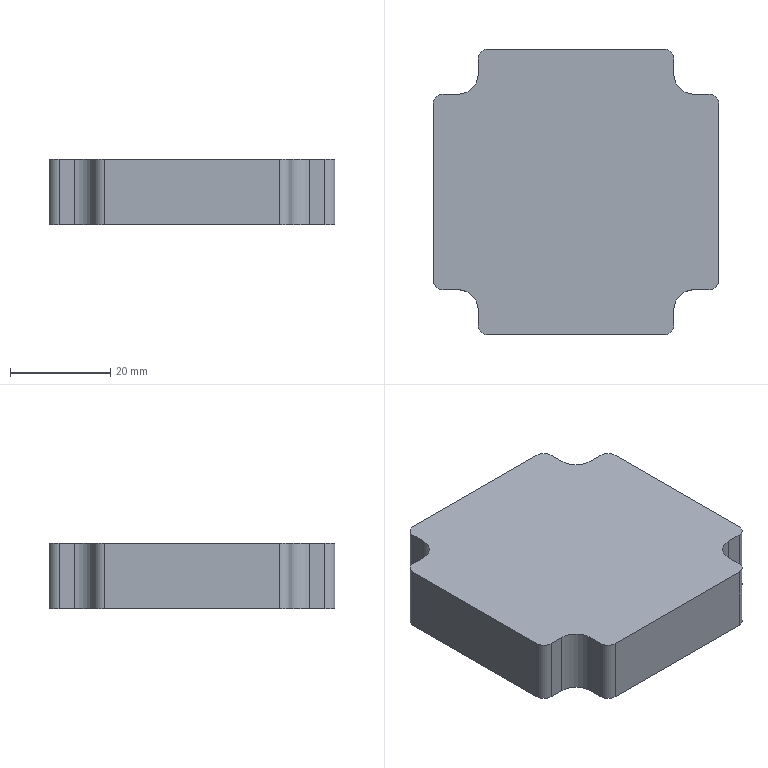Part | SolidWorks | features BaseBody 1 | 1 solid | 41 faces | box 57 x 57 x 13 mm | volume 37451 mm3 | cylinder 22 | plane 19 | commonest cylinder face diameters 3 x8 4 x8 8 x4 10 x2
STEP:
#1=CARTESIAN_POINT('',(5.,0.,7.));
#2=VERTEX_POINT('',#1);
#3=CARTESIAN_POINT('',(-5.,0.,7.));
#4=VERTEX_POINT('',#3);
#5=CARTESIAN_POINT('',(0.,0.,7.));
#6=DIRECTION('',(0.,0.,-1.));
#7=DIRECTION('',(-1.,0.,0.));
#8=AXIS2_PLACEMENT_3D('',#5,#6,#7);
#9=CIRCLE('',#8,5.);
#10=EDGE_CURVE('',#2,#4,#9,.T.);
#11=ORIENTED_EDGE('',*,*,#10,.F.);
#12=CARTESIAN_POINT('',(5.,0.,0.));
#13=VERTEX_POINT('',#12);
#14=CARTESIAN_POINT('',(5.,0.,7.));
#15=DIRECTION('',(0.,0.,-1.));
#16=VECTOR('',#15,1000.);
#17=LINE('',#14,#16);
#18=EDGE_CURVE('',#2,#13,#17,.T.);
#19=ORIENTED_EDGE('',*,*,#18,.T.);
#20=CARTESIAN_POINT('',(-5.,0.,0.));
#21=VERTEX_POINT('',#20);
#22=CARTESIAN_POINT('',(0.,0.,0.));
#23=DIRECTION('',(0.,0.,-1.));
#24=DIRECTION('',(-1.,0.,0.));
#25=AXIS2_PLACEMENT_3D('',#22,#23,#24);
#26=CIRCLE('',#25,5.);
#27=EDGE_CURVE('',#13,#21,#26,.T.);
#28=ORIENTED_EDGE('',*,*,#27,.T.);
#29=CARTESIAN_POINT('',(-5.,0.,7.));
#30=DIRECTION('',(0.,0.,-1.));
#31=VECTOR('',#30,1000.);
#32=LINE('',#29,#31);
#33=EDGE_CURVE('',#4,#21,#32,.T.);
#34=ORIENTED_EDGE('',*,*,#33,.F.);
#35=EDGE_LOOP('',(#11,#19,#28,#34));
#36=FACE_OUTER_BOUND('',#35,.T.);
#37=CARTESIAN_POINT('',(0.,0.,7.));
#38=DIRECTION('',(0.,0.,-1.));
#39=DIRECTION('',(-1.,0.,0.));
#40=AXIS2_PLACEMENT_3D('',#37,#38,#39);
#41=CYLINDRICAL_SURFACE('',#40,5.);
#42=ADVANCED_FACE('',(#36),#41,.F.);
#43=CARTESIAN_POINT('',(-24.,-16.5,4.));
#44=VERTEX_POINT('',#43);
#45=CARTESIAN_POINT('',(-27.,-16.5,4.));
#46=VERTEX_POINT('',#45);
#47=CARTESIAN_POINT('',(-25.5,-16.5,4.));
#48=DIRECTION('',(0.,0.,-1.));
#49=DIRECTION('',(-1.,0.,0.));
#50=AXIS2_PLACEMENT_3D('',#47,#48,#49);
#51=CIRCLE('',#50,1.5);
#52=EDGE_CURVE('',#44,#46,#51,.T.);
#53=ORIENTED_EDGE('',*,*,#52,.F.);
#54=CARTESIAN_POINT('',(-24.,-16.5,0.));
#55=VERTEX_POINT('',#54);
#56=CARTESIAN_POINT('',(-24.,-16.5,4.));
#57=DIRECTION('',(0.,0.,-1.));
#58=VECTOR('',#57,1000.);
#59=LINE('',#56,#58);
#60=EDGE_CURVE('',#44,#55,#59,.T.);
#61=ORIENTED_EDGE('',*,*,#60,.T.);
#62=CARTESIAN_POINT('',(-27.,-16.5,0.));
#63=VERTEX_POINT('',#62);
#64=CARTESIAN_POINT('',(-25.5,-16.5,0.));
#65=DIRECTION('',(0.,0.,-1.));
#66=DIRECTION('',(-1.,0.,0.));
#67=AXIS2_PLACEMENT_3D('',#64,#65,#66);
#68=CIRCLE('',#67,1.5);
#69=EDGE_CURVE('',#55,#63,#68,.T.);
#70=ORIENTED_EDGE('',*,*,#69,.T.);
#71=CARTESIAN_POINT('',(-27.,-16.5,4.));
#72=DIRECTION('',(0.,0.,-1.));
#73=VECTOR('',#72,1000.);
#74=LINE('',#71,#73);
#75=EDGE_CURVE('',#46,#63,#74,.T.);
#76=ORIENTED_EDGE('',*,*,#75,.F.);
#77=EDGE_LOOP('',(#53,#61,#70,#76));
#78=FACE_OUTER_BOUND('',#77,.T.);
#79=CARTESIAN_POINT('',(-25.5,-16.5,4.));
#80=DIRECTION('',(0.,0.,-1.));
#81=DIRECTION('',(-1.,0.,0.));
#82=AXIS2_PLACEMENT_3D('',#79,#80,#81);
#83=CYLINDRICAL_SURFACE('',#82,1.5);
#84=ADVANCED_FACE('',(#78),#83,.F.);
#85=CARTESIAN_POINT('',(-15.,25.5,4.));
#86=VERTEX_POINT('',#85);
#87=CARTESIAN_POINT('',(-18.,25.5,4.));
#88=VERTEX_POINT('',#87);
#89=CARTESIAN_POINT('',(-16.5,25.5,4.));
#90=DIRECTION('',(0.,0.,-1.));
#91=DIRECTION('',(-1.,0.,0.));
#92=AXIS2_PLACEMENT_3D('',#89,#90,#91);
#93=CIRCLE('',#92,1.5);
#94=EDGE_CURVE('',#86,#88,#93,.T.);
#95=ORIENTED_EDGE('',*,*,#94,.F.);
#96=CARTESIAN_POINT('',(-15.,25.5,0.));
#97=VERTEX_POINT('',#96);
#98=CARTESIAN_POINT('',(-15.,25.5,4.));
#99=DIRECTION('',(0.,0.,-1.));
#100=VECTOR('',#99,1000.);
#101=LINE('',#98,#100);
#102=EDGE_CURVE('',#86,#97,#101,.T.);
#103=ORIENTED_EDGE('',*,*,#102,.T.);
#104=CARTESIAN_POINT('',(-18.,25.5,0.));
#105=VERTEX_POINT('',#104);
#106=CARTESIAN_POINT('',(-16.5,25.5,0.));
#107=DIRECTION('',(0.,0.,-1.));
#108=DIRECTION('',(-1.,0.,0.));
#109=AXIS2_PLACEMENT_3D('',#106,#107,#108);
#110=CIRCLE('',#109,1.5);
#111=EDGE_CURVE('',#97,#105,#110,.T.);
#112=ORIENTED_EDGE('',*,*,#111,.T.);
#113=CARTESIAN_POINT('',(-18.,25.5,4.));
#114=DIRECTION('',(0.,0.,-1.));
#115=VECTOR('',#114,1000.);
#116=LINE('',#113,#115);
#117=EDGE_CURVE('',#88,#105,#116,.T.);
#118=ORIENTED_EDGE('',*,*,#117,.F.);
#119=EDGE_LOOP('',(#95,#103,#112,#118));
#120=FACE_OUTER_BOUND('',#119,.T.);
#121=CARTESIAN_POINT('',(-16.5,25.5,4.));
#122=DIRECTION('',(0.,0.,-1.));
#123=DIRECTION('',(-1.,0.,0.));
#124=AXIS2_PLACEMENT_3D('',#121,#122,#123);
#125=CYLINDRICAL_SURFACE('',#124,1.5);
#126=ADVANCED_FACE('',(#120),#125,.F.);
#127=CARTESIAN_POINT('',(27.,16.5,4.));
#128=VERTEX_POINT('',#127);
#129=CARTESIAN_POINT('',(24.,16.5,4.));
#130=VERTEX_POINT('',#129);
#131=CARTESIAN_POINT('',(25.5,16.5,4.));
#132=DIRECTION('',(0.,0.,-1.));
#133=DIRECTION('',(-1.,0.,0.));
#134=AXIS2_PLACEMENT_3D('',#131,#132,#133);
#135=CIRCLE('',#134,1.5);
#136=EDGE_CURVE('',#128,#130,#135,.T.);
#137=ORIENTED_EDGE('',*,*,#136,.F.);
#138=CARTESIAN_POINT('',(27.,16.5,0.));
#139=VERTEX_POINT('',#138);
#140=CARTESIAN_POINT('',(27.,16.5,4.));
#141=DIRECTION('',(0.,0.,-1.));
#142=VECTOR('',#141,1000.);
#143=LINE('',#140,#142);
#144=EDGE_CURVE('',#128,#139,#143,.T.);
#145=ORIENTED_EDGE('',*,*,#144,.T.);
#146=CARTESIAN_POINT('',(24.,16.5,0.));
#147=VERTEX_POINT('',#146);
#148=CARTESIAN_POINT('',(25.5,16.5,0.));
#149=DIRECTION('',(0.,0.,-1.));
#150=DIRECTION('',(-1.,0.,0.));
#151=AXIS2_PLACEMENT_3D('',#148,#149,#150);
#152=CIRCLE('',#151,1.5);
#153=EDGE_CURVE('',#139,#147,#152,.T.);
#154=ORIENTED_EDGE('',*,*,#153,.T.);
#155=CARTESIAN_POINT('',(24.,16.5,4.));
#156=DIRECTION('',(0.,0.,-1.));
#157=VECTOR('',#156,1000.);
#158=LINE('',#155,#157);
#159=EDGE_CURVE('',#130,#147,#158,.T.);
#160=ORIENTED_EDGE('',*,*,#159,.F.);
#161=EDGE_LOOP('',(#137,#145,#154,#160));
#162=FACE_OUTER_BOUND('',#161,.T.);
#163=CARTESIAN_POINT('',(25.5,16.5,4.));
#164=DIRECTION('',(0.,0.,-1.));
#165=DIRECTION('',(-1.,0.,0.));
#166=AXIS2_PLACEMENT_3D('',#163,#164,#165);
#167=CYLINDRICAL_SURFACE('',#166,1.5);
#168=ADVANCED_FACE('',(#162),#167,.F.);
#169=CARTESIAN_POINT('',(18.,-25.5,4.));
#170=VERTEX_POINT('',#169);
#171=CARTESIAN_POINT('',(15.,-25.5,4.));
#172=VERTEX_POINT('',#171);
#173=CARTESIAN_POINT('',(16.5,-25.5,4.));
#174=DIRECTION('',(0.,0.,-1.));
#175=DIRECTION('',(-1.,0.,0.));
#176=AXIS2_PLACEMENT_3D('',#173,#174,#175);
#177=CIRCLE('',#176,1.5);
#178=EDGE_CURVE('',#170,#172,#177,.T.);
#179=ORIENTED_EDGE('',*,*,#178,.F.);
#180=CARTESIAN_POINT('',(18.,-25.5,0.));
#181=VERTEX_POINT('',#180);
#182=CARTESIAN_POINT('',(18.,-25.5,4.));
#183=DIRECTION('',(0.,0.,-1.));
#184=VECTOR('',#183,1000.);
#185=LINE('',#182,#184);
#186=EDGE_CURVE('',#170,#181,#185,.T.);
#187=ORIENTED_EDGE('',*,*,#186,.T.);
#188=CARTESIAN_POINT('',(15.,-25.5,0.));
#189=VERTEX_POINT('',#188);
#190=CARTESIAN_POINT('',(16.5,-25.5,0.));
#191=DIRECTION('',(0.,0.,-1.));
#192=DIRECTION('',(-1.,0.,0.));
#193=AXIS2_PLACEMENT_3D('',#190,#191,#192);
#194=CIRCLE('',#193,1.5);
#195=EDGE_CURVE('',#181,#189,#194,.T.);
#196=ORIENTED_EDGE('',*,*,#195,.T.);
#197=CARTESIAN_POINT('',(15.,-25.5,4.));
#198=DIRECTION('',(0.,0.,-1.));
#199=VECTOR('',#198,1000.);
#200=LINE('',#197,#199);
#201=EDGE_CURVE('',#172,#189,#200,.T.);
#202=ORIENTED_EDGE('',*,*,#201,.F.);
#203=EDGE_LOOP('',(#179,#187,#196,#202));
#204=FACE_OUTER_BOUND('',#203,.T.);
#205=CARTESIAN_POINT('',(16.5,-25.5,4.));
#206=DIRECTION('',(0.,0.,-1.));
#207=DIRECTION('',(-1.,0.,0.));
#208=AXIS2_PLACEMENT_3D('',#205,#206,#207);
#209=CYLINDRICAL_SURFACE('',#208,1.5);
#210=ADVANCED_FACE('',(#204),#209,.F.);
#211=CARTESIAN_POINT('',(19.5,26.5,0.));
#212=VERTEX_POINT('',#211);
#213=CARTESIAN_POINT('',(17.5,28.5,0.));
#214=VERTEX_POINT('',#213);
#215=CARTESIAN_POINT('',(17.5,26.5,0.));
#216=DIRECTION('',(0.,0.,1.));
#217=DIRECTION('',(-1.,0.,0.));
#218=AXIS2_PLACEMENT_3D('',#215,#216,#217);
#219=CIRCLE('',#218,2.);
#220=EDGE_CURVE('',#212,#214,#219,.T.);
#221=ORIENTED_EDGE('',*,*,#220,.T.);
#222=CARTESIAN_POINT('',(17.5,28.5,13.));
#223=VERTEX_POINT('',#222);
#224=CARTESIAN_POINT('',(17.5,28.5,13.));
#225=DIRECTION('',(0.,0.,-1.));
#226=VECTOR('',#225,1000.);
#227=LINE('',#224,#226);
#228=EDGE_CURVE('',#223,#214,#227,.T.);
#229=ORIENTED_EDGE('',*,*,#228,.F.);
#230=CARTESIAN_POINT('',(19.5,26.5,13.));
#231=VERTEX_POINT('',#230);
#232=CARTESIAN_POINT('',(17.5,26.5,13.));
#233=DIRECTION('',(0.,0.,1.));
#234=DIRECTION('',(-1.,0.,0.));
#235=AXIS2_PLACEMENT_3D('',#232,#233,#234);
#236=CIRCLE('',#235,2.);
#237=EDGE_CURVE('',#231,#223,#236,.T.);
#238=ORIENTED_EDGE('',*,*,#237,.F.);
#239=CARTESIAN_POINT('',(19.5,26.5,13.));
#240=DIRECTION('',(0.,0.,-1.));
#241=VECTOR('',#240,1000.);
#242=LINE('',#239,#241);
#243=EDGE_CURVE('',#231,#212,#242,.T.);
#244=ORIENTED_EDGE('',*,*,#243,.T.);
#245=EDGE_LOOP('',(#221,#229,#238,#244));
#246=FACE_OUTER_BOUND('',#245,.T.);
#247=CARTESIAN_POINT('',(17.5,26.5,13.));
#248=DIRECTION('',(0.,0.,-1.));
#249=DIRECTION('',(-1.,0.,0.));
#250=AXIS2_PLACEMENT_3D('',#247,#248,#249);
#251=CYLINDRICAL_SURFACE('',#250,2.);
#252=ADVANCED_FACE('',(#246),#251,.T.);
#253=CARTESIAN_POINT('',(-17.5,28.5,0.));
#254=VERTEX_POINT('',#253);
#255=CARTESIAN_POINT('',(-17.5,28.5,0.));
#256=DIRECTION('',(-1.,0.,0.));
#257=VECTOR('',#256,1000.);
#258=LINE('',#255,#257);
#259=EDGE_CURVE('',#214,#254,#258,.T.);
#260=ORIENTED_EDGE('',*,*,#259,.T.);
#261=CARTESIAN_POINT('',(-17.5,28.5,13.));
#262=VERTEX_POINT('',#261);
#263=CARTESIAN_POINT('',(-17.5,28.5,13.));
#264=DIRECTION('',(0.,0.,-1.));
#265=VECTOR('',#264,1000.);
#266=LINE('',#263,#265);
#267=EDGE_CURVE('',#262,#254,#266,.T.);
#268=ORIENTED_EDGE('',*,*,#267,.F.);
#269=CARTESIAN_POINT('',(-17.5,28.5,13.));
#270=DIRECTION('',(-1.,0.,0.));
#271=VECTOR('',#270,1000.);
#272=LINE('',#269,#271);
#273=EDGE_CURVE('',#223,#262,#272,.T.);
#274=ORIENTED_EDGE('',*,*,#273,.F.);
#275=ORIENTED_EDGE('',*,*,#228,.T.);
#276=EDGE_LOOP('',(#260,#268,#274,#275));
#277=FACE_OUTER_BOUND('',#276,.T.);
#278=CARTESIAN_POINT('',(-17.5,28.5,13.));
#279=DIRECTION('',(0.,-1.,0.));
#280=DIRECTION('',(0.,0.,-1.));
#281=AXIS2_PLACEMENT_3D('',#278,#279,#280);
#282=PLANE('',#281);
#283=ADVANCED_FACE('',(#277),#282,.F.);
#284=CARTESIAN_POINT('',(-19.5,26.5,0.));
#285=VERTEX_POINT('',#284);
#286=CARTESIAN_POINT('',(-17.5,26.5,0.));
#287=DIRECTION('',(0.,0.,1.));
#288=DIRECTION('',(-1.,0.,0.));
#289=AXIS2_PLACEMENT_3D('',#286,#287,#288);
#290=CIRCLE('',#289,2.);
#291=EDGE_CURVE('',#254,#285,#290,.T.);
#292=ORIENTED_EDGE('',*,*,#291,.T.);
#293=CARTESIAN_POINT('',(-19.5,26.5,13.));
#294=VERTEX_POINT('',#293);
#295=CARTESIAN_POINT('',(-19.5,26.5,13.));
#296=DIRECTION('',(0.,0.,-1.));
#297=VECTOR('',#296,1000.);
#298=LINE('',#295,#297);
#299=EDGE_CURVE('',#294,#285,#298,.T.);
#300=ORIENTED_EDGE('',*,*,#299,.F.);
#301=CARTESIAN_POINT('',(-17.5,26.5,13.));
#302=DIRECTION('',(0.,0.,1.));
#303=DIRECTION('',(-1.,0.,0.));
#304=AXIS2_PLACEMENT_3D('',#301,#302,#303);
#305=CIRCLE('',#304,2.);
#306=EDGE_CURVE('',#262,#294,#305,.T.);
#307=ORIENTED_EDGE('',*,*,#306,.F.);
#308=ORIENTED_EDGE('',*,*,#267,.T.);
#309=EDGE_LOOP('',(#292,#300,#307,#308));
#310=FACE_OUTER_BOUND('',#309,.T.);
#311=CARTESIAN_POINT('',(-17.5,26.5,13.));
#312=DIRECTION('',(0.,0.,-1.));
#313=DIRECTION('',(-1.,0.,0.));
#314=AXIS2_PLACEMENT_3D('',#311,#312,#313);
#315=CYLINDRICAL_SURFACE('',#314,2.);
#316=ADVANCED_FACE('',(#310),#315,.T.);
#317=CARTESIAN_POINT('',(-19.5,23.5,0.));
#318=VERTEX_POINT('',#317);
#319=CARTESIAN_POINT('',(-19.5,23.5,0.));
#320=DIRECTION('',(0.,-1.,0.));
#321=VECTOR('',#320,1000.);
#322=LINE('',#319,#321);
#323=EDGE_CURVE('',#285,#318,#322,.T.);
#324=ORIENTED_EDGE('',*,*,#323,.T.);
#325=CARTESIAN_POINT('',(-19.5,23.5,13.));
#326=VERTEX_POINT('',#325);
#327=CARTESIAN_POINT('',(-19.5,23.5,13.));
#328=DIRECTION('',(0.,0.,-1.));
#329=VECTOR('',#328,1000.);
#330=LINE('',#327,#329);
#331=EDGE_CURVE('',#326,#318,#330,.T.);
#332=ORIENTED_EDGE('',*,*,#331,.F.);
#333=CARTESIAN_POINT('',(-19.5,23.5,13.));
#334=DIRECTION('',(0.,-1.,0.));
#335=VECTOR('',#334,1000.);
#336=LINE('',#333,#335);
#337=EDGE_CURVE('',#294,#326,#336,.T.);
#338=ORIENTED_EDGE('',*,*,#337,.F.);
#339=ORIENTED_EDGE('',*,*,#299,.T.);
#340=EDGE_LOOP('',(#324,#332,#338,#339));
#341=FACE_OUTER_BOUND('',#340,.T.);
#342=CARTESIAN_POINT('',(-19.5,23.5,13.));
#343=DIRECTION('',(1.,0.,0.));
#344=DIRECTION('',(0.,1.,0.));
#345=AXIS2_PLACEMENT_3D('',#342,#343,#344);
#346=PLANE('',#345);
#347=ADVANCED_FACE('',(#341),#346,.F.);
#348=CARTESIAN_POINT('',(-23.5,19.5,0.));
#349=VERTEX_POINT('',#348);
#350=CARTESIAN_POINT('',(-23.5,23.5,0.));
#351=DIRECTION('',(0.,0.,-1.));
#352=DIRECTION('',(1.,0.,0.));
#353=AXIS2_PLACEMENT_3D('',#350,#351,#352);
#354=CIRCLE('',#353,4.);
#355=EDGE_CURVE('',#318,#349,#354,.T.);
#356=ORIENTED_EDGE('',*,*,#355,.T.);
#357=CARTESIAN_POINT('',(-23.5,19.5,13.));
#358=VERTEX_POINT('',#357);
#359=CARTESIAN_POINT('',(-23.5,19.5,13.));
#360=DIRECTION('',(0.,0.,-1.));
#361=VECTOR('',#360,1000.);
#362=LINE('',#359,#361);
#363=EDGE_CURVE('',#358,#349,#362,.T.);
#364=ORIENTED_EDGE('',*,*,#363,.F.);
#365=CARTESIAN_POINT('',(-23.5,23.5,13.));
#366=DIRECTION('',(0.,0.,-1.));
#367=DIRECTION('',(1.,0.,0.));
#368=AXIS2_PLACEMENT_3D('',#365,#366,#367);
#369=CIRCLE('',#368,4.);
#370=EDGE_CURVE('',#326,#358,#369,.T.);
#371=ORIENTED_EDGE('',*,*,#370,.F.);
#372=ORIENTED_EDGE('',*,*,#331,.T.);
#373=EDGE_LOOP('',(#356,#364,#371,#372));
#374=FACE_OUTER_BOUND('',#373,.T.);
#375=CARTESIAN_POINT('',(-23.5,23.5,13.));
#376=DIRECTION('',(0.,0.,-1.));
#377=DIRECTION('',(-1.,0.,0.));
#378=AXIS2_PLACEMENT_3D('',#375,#376,#377);
#379=CYLINDRICAL_SURFACE('',#378,4.);
#380=ADVANCED_FACE('',(#374),#379,.F.);
#381=CARTESIAN_POINT('',(-26.5,19.5,0.));
#382=VERTEX_POINT('',#381);
#383=CARTESIAN_POINT('',(-26.5,19.5,0.));
#384=DIRECTION('',(-1.,0.,0.));
#385=VECTOR('',#384,1000.);
#386=LINE('',#383,#385);
#387=EDGE_CURVE('',#349,#382,#386,.T.);
#388=ORIENTED_EDGE('',*,*,#387,.T.);
#389=CARTESIAN_POINT('',(-26.5,19.5,13.));
#390=VERTEX_POINT('',#389);
#391=CARTESIAN_POINT('',(-26.5,19.5,13.));
#392=DIRECTION('',(0.,0.,-1.));
#393=VECTOR('',#392,1000.);
#394=LINE('',#391,#393);
#395=EDGE_CURVE('',#390,#382,#394,.T.);
#396=ORIENTED_EDGE('',*,*,#395,.F.);
#397=CARTESIAN_POINT('',(-26.5,19.5,13.));
#398=DIRECTION('',(-1.,0.,0.));
#399=VECTOR('',#398,1000.);
#400=LINE('',#397,#399);
#401=EDGE_CURVE('',#358,#390,#400,.T.);
#402=ORIENTED_EDGE('',*,*,#401,.F.);
#403=ORIENTED_EDGE('',*,*,#363,.T.);
#404=EDGE_LOOP('',(#388,#396,#402,#403));
#405=FACE_OUTER_BOUND('',#404,.T.);
#406=CARTESIAN_POINT('',(-26.5,19.5,13.));
#407=DIRECTION('',(0.,-1.,0.));
#408=DIRECTION('',(0.,0.,-1.));
#409=AXIS2_PLACEMENT_3D('',#406,#407,#408);
#410=PLANE('',#409);
#411=ADVANCED_FACE('',(#405),#410,.F.);
#412=CARTESIAN_POINT('',(-28.5,17.5,0.));
#413=VERTEX_POINT('',#412);
#414=CARTESIAN_POINT('',(-26.5,17.5,0.));
#415=DIRECTION('',(0.,0.,1.));
#416=DIRECTION('',(-1.,0.,0.));
#417=AXIS2_PLACEMENT_3D('',#414,#415,#416);
#418=CIRCLE('',#417,2.);
#419=EDGE_CURVE('',#382,#413,#418,.T.);
#420=ORIENTED_EDGE('',*,*,#419,.T.);
#421=CARTESIAN_POINT('',(-28.5,17.5,13.));
#422=VERTEX_POINT('',#421);
#423=CARTESIAN_POINT('',(-28.5,17.5,13.));
#424=DIRECTION('',(0.,0.,-1.));
#425=VECTOR('',#424,1000.);
#426=LINE('',#423,#425);
#427=EDGE_CURVE('',#422,#413,#426,.T.);
#428=ORIENTED_EDGE('',*,*,#427,.F.);
#429=CARTESIAN_POINT('',(-26.5,17.5,13.));
#430=DIRECTION('',(0.,0.,1.));
#431=DIRECTION('',(-1.,0.,0.));
#432=AXIS2_PLACEMENT_3D('',#429,#430,#431);
#433=CIRCLE('',#432,2.);
#434=EDGE_CURVE('',#390,#422,#433,.T.);
#435=ORIENTED_EDGE('',*,*,#434,.F.);
#436=ORIENTED_EDGE('',*,*,#395,.T.);
#437=EDGE_LOOP('',(#420,#428,#435,#436));
#438=FACE_OUTER_BOUND('',#437,.T.);
#439=CARTESIAN_POINT('',(-26.5,17.5,13.));
#440=DIRECTION('',(0.,0.,-1.));
#441=DIRECTION('',(-1.,0.,0.));
#442=AXIS2_PLACEMENT_3D('',#439,#440,#441);
#443=CYLINDRICAL_SURFACE('',#442,2.);
#444=ADVANCED_FACE('',(#438),#443,.T.);
#445=CARTESIAN_POINT('',(-28.5,-17.5,0.));
#446=VERTEX_POINT('',#445);
#447=CARTESIAN_POINT('',(-28.5,-17.5,0.));
#448=DIRECTION('',(0.,-1.,0.));
#449=VECTOR('',#448,1000.);
#450=LINE('',#447,#449);
#451=EDGE_CURVE('',#413,#446,#450,.T.);
#452=ORIENTED_EDGE('',*,*,#451,.T.);
#453=CARTESIAN_POINT('',(-28.5,-17.5,13.));
#454=VERTEX_POINT('',#453);
#455=CARTESIAN_POINT('',(-28.5,-17.5,13.));
#456=DIRECTION('',(0.,0.,-1.));
#457=VECTOR('',#456,1000.);
#458=LINE('',#455,#457);
#459=EDGE_CURVE('',#454,#446,#458,.T.);
#460=ORIENTED_EDGE('',*,*,#459,.F.);
#461=CARTESIAN_POINT('',(-28.5,-17.5,13.));
#462=DIRECTION('',(0.,-1.,0.));
#463=VECTOR('',#462,1000.);
#464=LINE('',#461,#463);
#465=EDGE_CURVE('',#422,#454,#464,.T.);
#466=ORIENTED_EDGE('',*,*,#465,.F.);
#467=ORIENTED_EDGE('',*,*,#427,.T.);
#468=EDGE_LOOP('',(#452,#460,#466,#467));
#469=FACE_OUTER_BOUND('',#468,.T.);
#470=CARTESIAN_POINT('',(-28.5,-17.5,13.));
#471=DIRECTION('',(1.,0.,0.));
#472=DIRECTION('',(0.,1.,0.));
#473=AXIS2_PLACEMENT_3D('',#470,#471,#472);
#474=PLANE('',#473);
#475=ADVANCED_FACE('',(#469),#474,.F.);
#476=CARTESIAN_POINT('',(-26.5,-19.5,0.));
#477=VERTEX_POINT('',#476);
#478=CARTESIAN_POINT('',(-26.5,-17.5,0.));
#479=DIRECTION('',(0.,0.,1.));
#480=DIRECTION('',(-1.,0.,0.));
#481=AXIS2_PLACEMENT_3D('',#478,#479,#480);
#482=CIRCLE('',#481,2.);
#483=EDGE_CURVE('',#446,#477,#482,.T.);
#484=ORIENTED_EDGE('',*,*,#483,.T.);
#485=CARTESIAN_POINT('',(-26.5,-19.5,13.));
#486=VERTEX_POINT('',#485);
#487=CARTESIAN_POINT('',(-26.5,-19.5,13.));
#488=DIRECTION('',(0.,0.,-1.));
#489=VECTOR('',#488,1000.);
#490=LINE('',#487,#489);
#491=EDGE_CURVE('',#486,#477,#490,.T.);
#492=ORIENTED_EDGE('',*,*,#491,.F.);
#493=CARTESIAN_POINT('',(-26.5,-17.5,13.));
#494=DIRECTION('',(0.,0.,1.));
#495=DIRECTION('',(-1.,0.,0.));
#496=AXIS2_PLACEMENT_3D('',#493,#494,#495);
#497=CIRCLE('',#496,2.);
#498=EDGE_CURVE('',#454,#486,#497,.T.);
#499=ORIENTED_EDGE('',*,*,#498,.F.);
#500=ORIENTED_EDGE('',*,*,#459,.T.);
#501=EDGE_LOOP('',(#484,#492,#499,#500));
#502=FACE_OUTER_BOUND('',#501,.T.);
#503=CARTESIAN_POINT('',(-26.5,-17.5,13.));
#504=DIRECTION('',(0.,0.,-1.));
#505=DIRECTION('',(-1.,0.,0.));
#506=AXIS2_PLACEMENT_3D('',#503,#504,#505);
#507=CYLINDRICAL_SURFACE('',#506,2.);
#508=ADVANCED_FACE('',(#502),#507,.T.);
#509=CARTESIAN_POINT('',(-23.5,-19.5,0.));
#510=VERTEX_POINT('',#509);
#511=CARTESIAN_POINT('',(-23.5,-19.5,0.));
#512=DIRECTION('',(1.,0.,0.));
#513=VECTOR('',#512,1000.);
#514=LINE('',#511,#513);
#515=EDGE_CURVE('',#477,#510,#514,.T.);
#516=ORIENTED_EDGE('',*,*,#515,.T.);
#517=CARTESIAN_POINT('',(-23.5,-19.5,13.));
#518=VERTEX_POINT('',#517);
#519=CARTESIAN_POINT('',(-23.5,-19.5,13.));
#520=DIRECTION('',(0.,0.,-1.));
#521=VECTOR('',#520,1000.);
#522=LINE('',#519,#521);
#523=EDGE_CURVE('',#518,#510,#522,.T.);
#524=ORIENTED_EDGE('',*,*,#523,.F.);
#525=CARTESIAN_POINT('',(-23.5,-19.5,13.));
#526=DIRECTION('',(1.,0.,0.));
#527=VECTOR('',#526,1000.);
#528=LINE('',#525,#527);
#529=EDGE_CURVE('',#486,#518,#528,.T.);
#530=ORIENTED_EDGE('',*,*,#529,.F.);
#531=ORIENTED_EDGE('',*,*,#491,.T.);
#532=EDGE_LOOP('',(#516,#524,#530,#531));
#533=FACE_OUTER_BOUND('',#532,.T.);
#534=CARTESIAN_POINT('',(-23.5,-19.5,13.));
#535=DIRECTION('',(0.,1.,0.));
#536=DIRECTION('',(1.,0.,0.));
#537=AXIS2_PLACEMENT_3D('',#534,#535,#536);
#538=PLANE('',#537);
#539=ADVANCED_FACE('',(#533),#538,.F.);
#540=CARTESIAN_POINT('',(-19.5,-23.5,0.));
#541=VERTEX_POINT('',#540);
#542=CARTESIAN_POINT('',(-23.5,-23.5,0.));
#543=DIRECTION('',(0.,0.,-1.));
#544=DIRECTION('',(1.,0.,0.));
#545=AXIS2_PLACEMENT_3D('',#542,#543,#544);
#546=CIRCLE('',#545,4.);
#547=EDGE_CURVE('',#510,#541,#546,.T.);
#548=ORIENTED_EDGE('',*,*,#547,.T.);
#549=CARTESIAN_POINT('',(-19.5,-23.5,13.));
#550=VERTEX_POINT('',#549);
#551=CARTESIAN_POINT('',(-19.5,-23.5,13.));
#552=DIRECTION('',(0.,0.,-1.));
#553=VECTOR('',#552,1000.);
#554=LINE('',#551,#553);
#555=EDGE_CURVE('',#550,#541,#554,.T.);
#556=ORIENTED_EDGE('',*,*,#555,.F.);
#557=CARTESIAN_POINT('',(-23.5,-23.5,13.));
#558=DIRECTION('',(0.,0.,-1.));
#559=DIRECTION('',(1.,0.,0.));
#560=AXIS2_PLACEMENT_3D('',#557,#558,#559);
#561=CIRCLE('',#560,4.);
#562=EDGE_CURVE('',#518,#550,#561,.T.);
#563=ORIENTED_EDGE('',*,*,#562,.F.);
#564=ORIENTED_EDGE('',*,*,#523,.T.);
#565=EDGE_LOOP('',(#548,#556,#563,#564));
#566=FACE_OUTER_BOUND('',#565,.T.);
#567=CARTESIAN_POINT('',(-23.5,-23.5,13.));
#568=DIRECTION('',(0.,0.,-1.));
#569=DIRECTION('',(-1.,0.,0.));
#570=AXIS2_PLACEMENT_3D('',#567,#568,#569);
#571=CYLINDRICAL_SURFACE('',#570,4.);
#572=ADVANCED_FACE('',(#566),#571,.F.);
#573=CARTESIAN_POINT('',(-19.5,-26.5,0.));
#574=VERTEX_POINT('',#573);
#575=CARTESIAN_POINT('',(-19.5,-26.5,0.));
#576=DIRECTION('',(0.,-1.,0.));
#577=VECTOR('',#576,1000.);
#578=LINE('',#575,#577);
#579=EDGE_CURVE('',#541,#574,#578,.T.);
#580=ORIENTED_EDGE('',*,*,#579,.T.);
#581=CARTESIAN_POINT('',(-19.5,-26.5,13.));
#582=VERTEX_POINT('',#581);
#583=CARTESIAN_POINT('',(-19.5,-26.5,13.));
#584=DIRECTION('',(0.,0.,-1.));
#585=VECTOR('',#584,1000.);
#586=LINE('',#583,#585);
#587=EDGE_CURVE('',#582,#574,#586,.T.);
#588=ORIENTED_EDGE('',*,*,#587,.F.);
#589=CARTESIAN_POINT('',(-19.5,-26.5,13.));
#590=DIRECTION('',(0.,-1.,0.));
#591=VECTOR('',#590,1000.);
#592=LINE('',#589,#591);
#593=EDGE_CURVE('',#550,#582,#592,.T.);
#594=ORIENTED_EDGE('',*,*,#593,.F.);
#595=ORIENTED_EDGE('',*,*,#555,.T.);
#596=EDGE_LOOP('',(#580,#588,#594,#595));
#597=FACE_OUTER_BOUND('',#596,.T.);
#598=CARTESIAN_POINT('',(-19.5,-26.5,13.));
#599=DIRECTION('',(1.,0.,0.));
#600=DIRECTION('',(0.,1.,0.));
#601=AXIS2_PLACEMENT_3D('',#598,#599,#600);
#602=PLANE('',#601);
#603=ADVANCED_FACE('',(#597),#602,.F.);
#604=CARTESIAN_POINT('',(-17.5,-28.5,0.));
#605=VERTEX_POINT('',#604);
#606=CARTESIAN_POINT('',(-17.5,-26.5,0.));
#607=DIRECTION('',(0.,0.,1.));
#608=DIRECTION('',(-1.,0.,0.));
#609=AXIS2_PLACEMENT_3D('',#606,#607,#608);
#610=CIRCLE('',#609,2.);
#611=EDGE_CURVE('',#574,#605,#610,.T.);
#612=ORIENTED_EDGE('',*,*,#611,.T.);
#613=CARTESIAN_POINT('',(-17.5,-28.5,13.));
#614=VERTEX_POINT('',#613);
#615=CARTESIAN_POINT('',(-17.5,-28.5,13.));
#616=DIRECTION('',(0.,0.,-1.));
#617=VECTOR('',#616,1000.);
#618=LINE('',#615,#617);
#619=EDGE_CURVE('',#614,#605,#618,.T.);
#620=ORIENTED_EDGE('',*,*,#619,.F.);
#621=CARTESIAN_POINT('',(-17.5,-26.5,13.));
#622=DIRECTION('',(0.,0.,1.));
#623=DIRECTION('',(-1.,0.,0.));
#624=AXIS2_PLACEMENT_3D('',#621,#622,#623);
#625=CIRCLE('',#624,2.);
#626=EDGE_CURVE('',#582,#614,#625,.T.);
#627=ORIENTED_EDGE('',*,*,#626,.F.);
#628=ORIENTED_EDGE('',*,*,#587,.T.);
#629=EDGE_LOOP('',(#612,#620,#627,#628));
#630=FACE_OUTER_BOUND('',#629,.T.);
#631=CARTESIAN_POINT('',(-17.5,-26.5,13.));
#632=DIRECTION('',(0.,0.,-1.));
#633=DIRECTION('',(-1.,0.,0.));
#634=AXIS2_PLACEMENT_3D('',#631,#632,#633);
#635=CYLINDRICAL_SURFACE('',#634,2.);
#636=ADVANCED_FACE('',(#630),#635,.T.);
#637=CARTESIAN_POINT('',(17.5,-28.5,0.));
#638=VERTEX_POINT('',#637);
#639=CARTESIAN_POINT('',(17.5,-28.5,0.));
#640=DIRECTION('',(1.,0.,0.));
#641=VECTOR('',#640,1000.);
#642=LINE('',#639,#641);
#643=EDGE_CURVE('',#605,#638,#642,.T.);
#644=ORIENTED_EDGE('',*,*,#643,.T.);
#645=CARTESIAN_POINT('',(17.5,-28.5,13.));
#646=VERTEX_POINT('',#645);
#647=CARTESIAN_POINT('',(17.5,-28.5,13.));
#648=DIRECTION('',(0.,0.,-1.));
#649=VECTOR('',#648,1000.);
#650=LINE('',#647,#649);
#651=EDGE_CURVE('',#646,#638,#650,.T.);
#652=ORIENTED_EDGE('',*,*,#651,.F.);
#653=CARTESIAN_POINT('',(17.5,-28.5,13.));
#654=DIRECTION('',(1.,0.,0.));
#655=VECTOR('',#654,1000.);
#656=LINE('',#653,#655);
#657=EDGE_CURVE('',#614,#646,#656,.T.);
#658=ORIENTED_EDGE('',*,*,#657,.F.);
#659=ORIENTED_EDGE('',*,*,#619,.T.);
#660=EDGE_LOOP('',(#644,#652,#658,#659));
#661=FACE_OUTER_BOUND('',#660,.T.);
#662=CARTESIAN_POINT('',(17.5,-28.5,13.));
#663=DIRECTION('',(0.,1.,0.));
#664=DIRECTION('',(1.,0.,0.));
#665=AXIS2_PLACEMENT_3D('',#662,#663,#664);
#666=PLANE('',#665);
#667=ADVANCED_FACE('',(#661),#666,.F.);
#668=CARTESIAN_POINT('',(19.5,-26.5,0.));
#669=VERTEX_POINT('',#668);
#670=CARTESIAN_POINT('',(17.5,-26.5,0.));
#671=DIRECTION('',(0.,0.,1.));
#672=DIRECTION('',(-1.,0.,0.));
#673=AXIS2_PLACEMENT_3D('',#670,#671,#672);
#674=CIRCLE('',#673,2.);
#675=EDGE_CURVE('',#638,#669,#674,.T.);
#676=ORIENTED_EDGE('',*,*,#675,.T.);
#677=CARTESIAN_POINT('',(19.5,-26.5,13.));
#678=VERTEX_POINT('',#677);
#679=CARTESIAN_POINT('',(19.5,-26.5,13.));
#680=DIRECTION('',(0.,0.,-1.));
#681=VECTOR('',#680,1000.);
#682=LINE('',#679,#681);
#683=EDGE_CURVE('',#678,#669,#682,.T.);
#684=ORIENTED_EDGE('',*,*,#683,.F.);
#685=CARTESIAN_POINT('',(17.5,-26.5,13.));
#686=DIRECTION('',(0.,0.,1.));
#687=DIRECTION('',(-1.,0.,0.));
#688=AXIS2_PLACEMENT_3D('',#685,#686,#687);
#689=CIRCLE('',#688,2.);
#690=EDGE_CURVE('',#646,#678,#689,.T.);
#691=ORIENTED_EDGE('',*,*,#690,.F.);
#692=ORIENTED_EDGE('',*,*,#651,.T.);
#693=EDGE_LOOP('',(#676,#684,#691,#692));
#694=FACE_OUTER_BOUND('',#693,.T.);
#695=CARTESIAN_POINT('',(17.5,-26.5,13.));
#696=DIRECTION('',(0.,0.,-1.));
#697=DIRECTION('',(-1.,0.,0.));
#698=AXIS2_PLACEMENT_3D('',#695,#696,#697);
#699=CYLINDRICAL_SURFACE('',#698,2.);
#700=ADVANCED_FACE('',(#694),#699,.T.);
#701=CARTESIAN_POINT('',(19.5,-23.5,0.));
#702=VERTEX_POINT('',#701);
#703=CARTESIAN_POINT('',(19.5,-23.5,0.));
#704=DIRECTION('',(0.,1.,0.));
#705=VECTOR('',#704,1000.);
#706=LINE('',#703,#705);
#707=EDGE_CURVE('',#669,#702,#706,.T.);
#708=ORIENTED_EDGE('',*,*,#707,.T.);
#709=CARTESIAN_POINT('',(19.5,-23.5,13.));
#710=VERTEX_POINT('',#709);
#711=CARTESIAN_POINT('',(19.5,-23.5,13.));
#712=DIRECTION('',(0.,0.,-1.));
#713=VECTOR('',#712,1000.);
#714=LINE('',#711,#713);
#715=EDGE_CURVE('',#710,#702,#714,.T.);
#716=ORIENTED_EDGE('',*,*,#715,.F.);
#717=CARTESIAN_POINT('',(19.5,-23.5,13.));
#718=DIRECTION('',(0.,1.,0.));
#719=VECTOR('',#718,1000.);
#720=LINE('',#717,#719);
#721=EDGE_CURVE('',#678,#710,#720,.T.);
#722=ORIENTED_EDGE('',*,*,#721,.F.);
#723=ORIENTED_EDGE('',*,*,#683,.T.);
#724=EDGE_LOOP('',(#708,#716,#722,#723));
#725=FACE_OUTER_BOUND('',#724,.T.);
#726=CARTESIAN_POINT('',(19.5,-23.5,13.));
#727=DIRECTION('',(-1.,0.,0.));
#728=DIRECTION('',(0.,0.,1.));
#729=AXIS2_PLACEMENT_3D('',#726,#727,#728);
#730=PLANE('',#729);
#731=ADVANCED_FACE('',(#725),#730,.F.);
#732=CARTESIAN_POINT('',(23.5,-19.5,0.));
#733=VERTEX_POINT('',#732);
#734=CARTESIAN_POINT('',(23.5,-23.5,0.));
#735=DIRECTION('',(0.,0.,-1.));
#736=DIRECTION('',(-1.,0.,0.));
#737=AXIS2_PLACEMENT_3D('',#734,#735,#736);
#738=CIRCLE('',#737,4.);
#739=EDGE_CURVE('',#702,#733,#738,.T.);
#740=ORIENTED_EDGE('',*,*,#739,.T.);
#741=CARTESIAN_POINT('',(23.5,-19.5,13.));
#742=VERTEX_POINT('',#741);
#743=CARTESIAN_POINT('',(23.5,-19.5,13.));
#744=DIRECTION('',(0.,0.,-1.));
#745=VECTOR('',#744,1000.);
#746=LINE('',#743,#745);
#747=EDGE_CURVE('',#742,#733,#746,.T.);
#748=ORIENTED_EDGE('',*,*,#747,.F.);
#749=CARTESIAN_POINT('',(23.5,-23.5,13.));
#750=DIRECTION('',(0.,0.,-1.));
#751=DIRECTION('',(-1.,0.,0.));
#752=AXIS2_PLACEMENT_3D('',#749,#750,#751);
#753=CIRCLE('',#752,4.);
#754=EDGE_CURVE('',#710,#742,#753,.T.);
#755=ORIENTED_EDGE('',*,*,#754,.F.);
#756=ORIENTED_EDGE('',*,*,#715,.T.);
#757=EDGE_LOOP('',(#740,#748,#755,#756));
#758=FACE_OUTER_BOUND('',#757,.T.);
#759=CARTESIAN_POINT('',(23.5,-23.5,13.));
#760=DIRECTION('',(0.,0.,-1.));
#761=DIRECTION('',(-1.,0.,0.));
#762=AXIS2_PLACEMENT_3D('',#759,#760,#761);
#763=CYLINDRICAL_SURFACE('',#762,4.);
#764=ADVANCED_FACE('',(#758),#763,.F.);
#765=CARTESIAN_POINT('',(26.5,-19.5,0.));
#766=VERTEX_POINT('',#765);
#767=CARTESIAN_POINT('',(26.5,-19.5,0.));
#768=DIRECTION('',(1.,0.,0.));
#769=VECTOR('',#768,1000.);
#770=LINE('',#767,#769);
#771=EDGE_CURVE('',#733,#766,#770,.T.);
#772=ORIENTED_EDGE('',*,*,#771,.T.);
#773=CARTESIAN_POINT('',(26.5,-19.5,13.));
#774=VERTEX_POINT('',#773);
#775=CARTESIAN_POINT('',(26.5,-19.5,13.));
#776=DIRECTION('',(0.,0.,-1.));
#777=VECTOR('',#776,1000.);
#778=LINE('',#775,#777);
#779=EDGE_CURVE('',#774,#766,#778,.T.);
#780=ORIENTED_EDGE('',*,*,#779,.F.);
#781=CARTESIAN_POINT('',(26.5,-19.5,13.));
#782=DIRECTION('',(1.,0.,0.));
#783=VECTOR('',#782,1000.);
#784=LINE('',#781,#783);
#785=EDGE_CURVE('',#742,#774,#784,.T.);
#786=ORIENTED_EDGE('',*,*,#785,.F.);
#787=ORIENTED_EDGE('',*,*,#747,.T.);
#788=EDGE_LOOP('',(#772,#780,#786,#787));
#789=FACE_OUTER_BOUND('',#788,.T.);
#790=CARTESIAN_POINT('',(26.5,-19.5,13.));
#791=DIRECTION('',(0.,1.,0.));
#792=DIRECTION('',(1.,0.,0.));
#793=AXIS2_PLACEMENT_3D('',#790,#791,#792);
#794=PLANE('',#793);
#795=ADVANCED_FACE('',(#789),#794,.F.);
#796=CARTESIAN_POINT('',(28.5,-17.5,0.));
#797=VERTEX_POINT('',#796);
#798=CARTESIAN_POINT('',(26.5,-17.5,0.));
#799=DIRECTION('',(0.,0.,1.));
#800=DIRECTION('',(-1.,0.,0.));
#801=AXIS2_PLACEMENT_3D('',#798,#799,#800);
#802=CIRCLE('',#801,2.);
#803=EDGE_CURVE('',#766,#797,#802,.T.);
#804=ORIENTED_EDGE('',*,*,#803,.T.);
#805=CARTESIAN_POINT('',(28.5,-17.5,13.));
#806=VERTEX_POINT('',#805);
#807=CARTESIAN_POINT('',(28.5,-17.5,13.));
#808=DIRECTION('',(0.,0.,-1.));
#809=VECTOR('',#808,1000.);
#810=LINE('',#807,#809);
#811=EDGE_CURVE('',#806,#797,#810,.T.);
#812=ORIENTED_EDGE('',*,*,#811,.F.);
#813=CARTESIAN_POINT('',(26.5,-17.5,13.));
#814=DIRECTION('',(0.,0.,1.));
#815=DIRECTION('',(-1.,0.,0.));
#816=AXIS2_PLACEMENT_3D('',#813,#814,#815);
#817=CIRCLE('',#816,2.);
#818=EDGE_CURVE('',#774,#806,#817,.T.);
#819=ORIENTED_EDGE('',*,*,#818,.F.);
#820=ORIENTED_EDGE('',*,*,#779,.T.);
#821=EDGE_LOOP('',(#804,#812,#819,#820));
#822=FACE_OUTER_BOUND('',#821,.T.);
#823=CARTESIAN_POINT('',(26.5,-17.5,13.));
#824=DIRECTION('',(0.,0.,-1.));
#825=DIRECTION('',(-1.,0.,0.));
#826=AXIS2_PLACEMENT_3D('',#823,#824,#825);
#827=CYLINDRICAL_SURFACE('',#826,2.);
#828=ADVANCED_FACE('',(#822),#827,.T.);
#829=CARTESIAN_POINT('',(28.5,17.5,0.));
#830=VERTEX_POINT('',#829);
#831=CARTESIAN_POINT('',(28.5,17.5,0.));
#832=DIRECTION('',(0.,1.,0.));
#833=VECTOR('',#832,1000.);
#834=LINE('',#831,#833);
#835=EDGE_CURVE('',#797,#830,#834,.T.);
#836=ORIENTED_EDGE('',*,*,#835,.T.);
#837=CARTESIAN_POINT('',(28.5,17.5,13.));
#838=VERTEX_POINT('',#837);
#839=CARTESIAN_POINT('',(28.5,17.5,13.));
#840=DIRECTION('',(0.,0.,-1.));
#841=VECTOR('',#840,1000.);
#842=LINE('',#839,#841);
#843=EDGE_CURVE('',#838,#830,#842,.T.);
#844=ORIENTED_EDGE('',*,*,#843,.F.);
#845=CARTESIAN_POINT('',(28.5,17.5,13.));
#846=DIRECTION('',(0.,1.,0.));
#847=VECTOR('',#846,1000.);
#848=LINE('',#845,#847);
#849=EDGE_CURVE('',#806,#838,#848,.T.);
#850=ORIENTED_EDGE('',*,*,#849,.F.);
#851=ORIENTED_EDGE('',*,*,#811,.T.);
#852=EDGE_LOOP('',(#836,#844,#850,#851));
#853=FACE_OUTER_BOUND('',#852,.T.);
#854=CARTESIAN_POINT('',(28.5,17.5,13.));
#855=DIRECTION('',(-1.,0.,0.));
#856=DIRECTION('',(0.,1.,0.));
#857=AXIS2_PLACEMENT_3D('',#854,#855,#856);
#858=PLANE('',#857);
#859=ADVANCED_FACE('',(#853),#858,.F.);
#860=CARTESIAN_POINT('',(26.5,19.5,0.));
#861=VERTEX_POINT('',#860);
#862=CARTESIAN_POINT('',(26.5,17.5,0.));
#863=DIRECTION('',(0.,0.,1.));
#864=DIRECTION('',(-1.,0.,0.));
#865=AXIS2_PLACEMENT_3D('',#862,#863,#864);
#866=CIRCLE('',#865,2.);
#867=EDGE_CURVE('',#830,#861,#866,.T.);
#868=ORIENTED_EDGE('',*,*,#867,.T.);
#869=CARTESIAN_POINT('',(26.5,19.5,13.));
#870=VERTEX_POINT('',#869);
#871=CARTESIAN_POINT('',(26.5,19.5,13.));
#872=DIRECTION('',(0.,0.,-1.));
#873=VECTOR('',#872,1000.);
#874=LINE('',#871,#873);
#875=EDGE_CURVE('',#870,#861,#874,.T.);
#876=ORIENTED_EDGE('',*,*,#875,.F.);
#877=CARTESIAN_POINT('',(26.5,17.5,13.));
#878=DIRECTION('',(0.,0.,1.));
#879=DIRECTION('',(-1.,0.,0.));
#880=AXIS2_PLACEMENT_3D('',#877,#878,#879);
#881=CIRCLE('',#880,2.);
#882=EDGE_CURVE('',#838,#870,#881,.T.);
#883=ORIENTED_EDGE('',*,*,#882,.F.);
#884=ORIENTED_EDGE('',*,*,#843,.T.);
#885=EDGE_LOOP('',(#868,#876,#883,#884));
#886=FACE_OUTER_BOUND('',#885,.T.);
#887=CARTESIAN_POINT('',(26.5,17.5,13.));
#888=DIRECTION('',(0.,0.,-1.));
#889=DIRECTION('',(-1.,0.,0.));
#890=AXIS2_PLACEMENT_3D('',#887,#888,#889);
#891=CYLINDRICAL_SURFACE('',#890,2.);
#892=ADVANCED_FACE('',(#886),#891,.T.);
#893=CARTESIAN_POINT('',(23.5,19.5,0.));
#894=VERTEX_POINT('',#893);
#895=CARTESIAN_POINT('',(23.5,19.5,0.));
#896=DIRECTION('',(-1.,0.,0.));
#897=VECTOR('',#896,1000.);
#898=LINE('',#895,#897);
#899=EDGE_CURVE('',#861,#894,#898,.T.);
#900=ORIENTED_EDGE('',*,*,#899,.T.);
#901=CARTESIAN_POINT('',(23.5,19.5,13.));
#902=VERTEX_POINT('',#901);
#903=CARTESIAN_POINT('',(23.5,19.5,13.));
#904=DIRECTION('',(0.,0.,-1.));
#905=VECTOR('',#904,1000.);
#906=LINE('',#903,#905);
#907=EDGE_CURVE('',#902,#894,#906,.T.);
#908=ORIENTED_EDGE('',*,*,#907,.F.);
#909=CARTESIAN_POINT('',(23.5,19.5,13.));
#910=DIRECTION('',(-1.,0.,0.));
#911=VECTOR('',#910,1000.);
#912=LINE('',#909,#911);
#913=EDGE_CURVE('',#870,#902,#912,.T.);
#914=ORIENTED_EDGE('',*,*,#913,.F.);
#915=ORIENTED_EDGE('',*,*,#875,.T.);
#916=EDGE_LOOP('',(#900,#908,#914,#915));
#917=FACE_OUTER_BOUND('',#916,.T.);
#918=CARTESIAN_POINT('',(23.5,19.5,13.));
#919=DIRECTION('',(0.,-1.,0.));
#920=DIRECTION('',(0.,0.,-1.));
#921=AXIS2_PLACEMENT_3D('',#918,#919,#920);
#922=PLANE('',#921);
#923=ADVANCED_FACE('',(#917),#922,.F.);
#924=CARTESIAN_POINT('',(19.5,23.5,0.));
#925=VERTEX_POINT('',#924);
#926=CARTESIAN_POINT('',(23.5,23.5,0.));
#927=DIRECTION('',(0.,0.,-1.));
#928=DIRECTION('',(1.,0.,0.));
#929=AXIS2_PLACEMENT_3D('',#926,#927,#928);
#930=CIRCLE('',#929,4.);
#931=EDGE_CURVE('',#894,#925,#930,.T.);
#932=ORIENTED_EDGE('',*,*,#931,.T.);
#933=CARTESIAN_POINT('',(19.5,23.5,13.));
#934=VERTEX_POINT('',#933);
#935=CARTESIAN_POINT('',(19.5,23.5,13.));
#936=DIRECTION('',(0.,0.,-1.));
#937=VECTOR('',#936,1000.);
#938=LINE('',#935,#937);
#939=EDGE_CURVE('',#934,#925,#938,.T.);
#940=ORIENTED_EDGE('',*,*,#939,.F.);
#941=CARTESIAN_POINT('',(23.5,23.5,13.));
#942=DIRECTION('',(0.,0.,-1.));
#943=DIRECTION('',(1.,0.,0.));
#944=AXIS2_PLACEMENT_3D('',#941,#942,#943);
#945=CIRCLE('',#944,4.);
#946=EDGE_CURVE('',#902,#934,#945,.T.);
#947=ORIENTED_EDGE('',*,*,#946,.F.);
#948=ORIENTED_EDGE('',*,*,#907,.T.);
#949=EDGE_LOOP('',(#932,#940,#947,#948));
#950=FACE_OUTER_BOUND('',#949,.T.);
#951=CARTESIAN_POINT('',(23.5,23.5,13.));
#952=DIRECTION('',(0.,0.,-1.));
#953=DIRECTION('',(-1.,0.,0.));
#954=AXIS2_PLACEMENT_3D('',#951,#952,#953);
#955=CYLINDRICAL_SURFACE('',#954,4.);
#956=ADVANCED_FACE('',(#950),#955,.F.);
#957=CARTESIAN_POINT('',(19.5,26.5,0.));
#958=DIRECTION('',(0.,1.,0.));
#959=VECTOR('',#958,1000.);
#960=LINE('',#957,#959);
#961=EDGE_CURVE('',#925,#212,#960,.T.);
#962=ORIENTED_EDGE('',*,*,#961,.T.);
#963=ORIENTED_EDGE('',*,*,#243,.F.);
#964=CARTESIAN_POINT('',(19.5,26.5,13.));
#965=DIRECTION('',(0.,1.,0.));
#966=VECTOR('',#965,1000.);
#967=LINE('',#964,#966);
#968=EDGE_CURVE('',#934,#231,#967,.T.);
#969=ORIENTED_EDGE('',*,*,#968,.F.);
#970=ORIENTED_EDGE('',*,*,#939,.T.);
#971=EDGE_LOOP('',(#962,#963,#969,#970));
#972=FACE_OUTER_BOUND('',#971,.T.);
#973=CARTESIAN_POINT('',(19.5,26.5,13.));
#974=DIRECTION('',(-1.,0.,0.));
#975=DIRECTION('',(0.,0.,1.));
#976=AXIS2_PLACEMENT_3D('',#973,#974,#975);
#977=PLANE('',#976);
#978=ADVANCED_FACE('',(#972),#977,.F.);
#979=ORIENTED_EDGE('',*,*,#237,.T.);
#980=ORIENTED_EDGE('',*,*,#273,.T.);
#981=ORIENTED_EDGE('',*,*,#306,.T.);
#982=ORIENTED_EDGE('',*,*,#337,.T.);
#983=ORIENTED_EDGE('',*,*,#370,.T.);
#984=ORIENTED_EDGE('',*,*,#401,.T.);
#985=ORIENTED_EDGE('',*,*,#434,.T.);
#986=ORIENTED_EDGE('',*,*,#465,.T.);
#987=ORIENTED_EDGE('',*,*,#498,.T.);
#988=ORIENTED_EDGE('',*,*,#529,.T.);
#989=ORIENTED_EDGE('',*,*,#562,.T.);
#990=ORIENTED_EDGE('',*,*,#593,.T.);
#991=ORIENTED_EDGE('',*,*,#626,.T.);
#992=ORIENTED_EDGE('',*,*,#657,.T.);
#993=ORIENTED_EDGE('',*,*,#690,.T.);
#994=ORIENTED_EDGE('',*,*,#721,.T.);
#995=ORIENTED_EDGE('',*,*,#754,.T.);
#996=ORIENTED_EDGE('',*,*,#785,.T.);
#997=ORIENTED_EDGE('',*,*,#818,.T.);
#998=ORIENTED_EDGE('',*,*,#849,.T.);
#999=ORIENTED_EDGE('',*,*,#882,.T.);
#1000=ORIENTED_EDGE('',*,*,#913,.T.);
#1001=ORIENTED_EDGE('',*,*,#946,.T.);
#1002=ORIENTED_EDGE('',*,*,#968,.T.);
#1003=EDGE_LOOP('',(#979,#980,#981,#982,#983,#984,#985,#986,#987,#988,#989,#990,#991,#992,#993,#994,#995,#996,#997,#998,#999,#1000,#1001,#1002));
#1004=FACE_OUTER_BOUND('',#1003,.T.);
#1005=CARTESIAN_POINT('',(17.5,26.5,13.));
#1006=DIRECTION('',(0.,0.,-1.));
#1007=DIRECTION('',(0.,-1.,0.));
#1008=AXIS2_PLACEMENT_3D('',#1005,#1006,#1007);
#1009=PLANE('',#1008);
#1010=ADVANCED_FACE('',(#1004),#1009,.F.);
#1011=CARTESIAN_POINT('',(0.,0.,0.));
#1012=DIRECTION('',(0.,0.,-1.));
#1013=DIRECTION('',(-1.,0.,0.));
#1014=AXIS2_PLACEMENT_3D('',#1011,#1012,#1013);
#1015=CIRCLE('',#1014,5.);
#1016=EDGE_CURVE('',#21,#13,#1015,.T.);
#1017=ORIENTED_EDGE('',*,*,#1016,.F.);
#1018=ORIENTED_EDGE('',*,*,#27,.F.);
#1019=EDGE_LOOP('',(#1017,#1018));
#1020=FACE_BOUND('',#1019,.T.);
#1021=CARTESIAN_POINT('',(-25.5,-16.5,0.));
#1022=DIRECTION('',(0.,0.,-1.));
#1023=DIRECTION('',(-1.,0.,0.));
#1024=AXIS2_PLACEMENT_3D('',#1021,#1022,#1023);
#1025=CIRCLE('',#1024,1.5);
#1026=EDGE_CURVE('',#63,#55,#1025,.T.);
#1027=ORIENTED_EDGE('',*,*,#1026,.F.);
#1028=ORIENTED_EDGE('',*,*,#69,.F.);
#1029=EDGE_LOOP('',(#1027,#1028));
#1030=FACE_BOUND('',#1029,.T.);
#1031=CARTESIAN_POINT('',(-16.5,25.5,0.));
#1032=DIRECTION('',(0.,0.,-1.));
#1033=DIRECTION('',(-1.,0.,0.));
#1034=AXIS2_PLACEMENT_3D('',#1031,#1032,#1033);
#1035=CIRCLE('',#1034,1.5);
#1036=EDGE_CURVE('',#105,#97,#1035,.T.);
#1037=ORIENTED_EDGE('',*,*,#1036,.F.);
#1038=ORIENTED_EDGE('',*,*,#111,.F.);
#1039=EDGE_LOOP('',(#1037,#1038));
#1040=FACE_BOUND('',#1039,.T.);
#1041=CARTESIAN_POINT('',(25.5,16.5,0.));
#1042=DIRECTION('',(0.,0.,-1.));
#1043=DIRECTION('',(-1.,0.,0.));
#1044=AXIS2_PLACEMENT_3D('',#1041,#1042,#1043);
#1045=CIRCLE('',#1044,1.5);
#1046=EDGE_CURVE('',#147,#139,#1045,.T.);
#1047=ORIENTED_EDGE('',*,*,#1046,.F.);
#1048=ORIENTED_EDGE('',*,*,#153,.F.);
#1049=EDGE_LOOP('',(#1047,#1048));
#1050=FACE_BOUND('',#1049,.T.);
#1051=CARTESIAN_POINT('',(16.5,-25.5,0.));
#1052=DIRECTION('',(0.,0.,-1.));
#1053=DIRECTION('',(-1.,0.,0.));
#1054=AXIS2_PLACEMENT_3D('',#1051,#1052,#1053);
#1055=CIRCLE('',#1054,1.5);
#1056=EDGE_CURVE('',#189,#181,#1055,.T.);
#1057=ORIENTED_EDGE('',*,*,#1056,.F.);
#1058=ORIENTED_EDGE('',*,*,#195,.F.);
#1059=EDGE_LOOP('',(#1057,#1058));
#1060=FACE_BOUND('',#1059,.T.);
#1061=ORIENTED_EDGE('',*,*,#220,.F.);
#1062=ORIENTED_EDGE('',*,*,#961,.F.);
#1063=ORIENTED_EDGE('',*,*,#931,.F.);
#1064=ORIENTED_EDGE('',*,*,#899,.F.);
#1065=ORIENTED_EDGE('',*,*,#867,.F.);
#1066=ORIENTED_EDGE('',*,*,#835,.F.);
#1067=ORIENTED_EDGE('',*,*,#803,.F.);
#1068=ORIENTED_EDGE('',*,*,#771,.F.);
#1069=ORIENTED_EDGE('',*,*,#739,.F.);
#1070=ORIENTED_EDGE('',*,*,#707,.F.);
#1071=ORIENTED_EDGE('',*,*,#675,.F.);
#1072=ORIENTED_EDGE('',*,*,#643,.F.);
#1073=ORIENTED_EDGE('',*,*,#611,.F.);
#1074=ORIENTED_EDGE('',*,*,#579,.F.);
#1075=ORIENTED_EDGE('',*,*,#547,.F.);
#1076=ORIENTED_EDGE('',*,*,#515,.F.);
#1077=ORIENTED_EDGE('',*,*,#483,.F.);
#1078=ORIENTED_EDGE('',*,*,#451,.F.);
#1079=ORIENTED_EDGE('',*,*,#419,.F.);
#1080=ORIENTED_EDGE('',*,*,#387,.F.);
#1081=ORIENTED_EDGE('',*,*,#355,.F.);
#1082=ORIENTED_EDGE('',*,*,#323,.F.);
#1083=ORIENTED_EDGE('',*,*,#291,.F.);
#1084=ORIENTED_EDGE('',*,*,#259,.F.);
#1085=EDGE_LOOP('',(#1061,#1062,#1063,#1064,#1065,#1066,#1067,#1068,#1069,#1070,#1071,#1072,#1073,#1074,#1075,#1076,#1077,#1078,#1079,#1080,#1081,#1082,#1083,#1084));
#1086=FACE_OUTER_BOUND('',#1085,.T.);
#1087=CARTESIAN_POINT('',(17.5,26.5,0.));
#1088=DIRECTION('',(0.,0.,-1.));
#1089=DIRECTION('',(0.,-1.,0.));
#1090=AXIS2_PLACEMENT_3D('',#1087,#1088,#1089);
#1091=PLANE('',#1090);
#1092=ADVANCED_FACE('',(#1020,#1030,#1040,#1050,#1060,#1086),#1091,.T.);
#1093=ORIENTED_EDGE('',*,*,#186,.F.);
#1094=CARTESIAN_POINT('',(16.5,-25.5,4.));
#1095=DIRECTION('',(0.,0.,-1.));
#1096=DIRECTION('',(-1.,0.,0.));
#1097=AXIS2_PLACEMENT_3D('',#1094,#1095,#1096);
#1098=CIRCLE('',#1097,1.5);
#1099=EDGE_CURVE('',#172,#170,#1098,.T.);
#1100=ORIENTED_EDGE('',*,*,#1099,.F.);
#1101=ORIENTED_EDGE('',*,*,#201,.T.);
#1102=ORIENTED_EDGE('',*,*,#1056,.T.);
#1103=EDGE_LOOP('',(#1093,#1100,#1101,#1102));
#1104=FACE_OUTER_BOUND('',#1103,.T.);
#1105=CARTESIAN_POINT('',(16.5,-25.5,4.));
#1106=DIRECTION('',(0.,0.,-1.));
#1107=DIRECTION('',(-1.,0.,0.));
#1108=AXIS2_PLACEMENT_3D('',#1105,#1106,#1107);
#1109=CYLINDRICAL_SURFACE('',#1108,1.5);
#1110=ADVANCED_FACE('',(#1104),#1109,.F.);
#1111=ORIENTED_EDGE('',*,*,#1099,.T.);
#1112=ORIENTED_EDGE('',*,*,#178,.T.);
#1113=EDGE_LOOP('',(#1111,#1112));
#1114=FACE_OUTER_BOUND('',#1113,.T.);
#1115=CARTESIAN_POINT('',(16.5,-25.5,4.));
#1116=DIRECTION('',(0.,0.,-1.));
#1117=DIRECTION('',(0.,-1.,0.));
#1118=AXIS2_PLACEMENT_3D('',#1115,#1116,#1117);
#1119=PLANE('',#1118);
#1120=ADVANCED_FACE('',(#1114),#1119,.T.);
#1121=ORIENTED_EDGE('',*,*,#144,.F.);
#1122=CARTESIAN_POINT('',(25.5,16.5,4.));
#1123=DIRECTION('',(0.,0.,-1.));
#1124=DIRECTION('',(-1.,0.,0.));
#1125=AXIS2_PLACEMENT_3D('',#1122,#1123,#1124);
#1126=CIRCLE('',#1125,1.5);
#1127=EDGE_CURVE('',#130,#128,#1126,.T.);
#1128=ORIENTED_EDGE('',*,*,#1127,.F.);
#1129=ORIENTED_EDGE('',*,*,#159,.T.);
#1130=ORIENTED_EDGE('',*,*,#1046,.T.);
#1131=EDGE_LOOP('',(#1121,#1128,#1129,#1130));
#1132=FACE_OUTER_BOUND('',#1131,.T.);
#1133=CARTESIAN_POINT('',(25.5,16.5,4.));
#1134=DIRECTION('',(0.,0.,-1.));
#1135=DIRECTION('',(-1.,0.,0.));
#1136=AXIS2_PLACEMENT_3D('',#1133,#1134,#1135);
#1137=CYLINDRICAL_SURFACE('',#1136,1.5);
#1138=ADVANCED_FACE('',(#1132),#1137,.F.);
#1139=ORIENTED_EDGE('',*,*,#1127,.T.);
#1140=ORIENTED_EDGE('',*,*,#136,.T.);
#1141=EDGE_LOOP('',(#1139,#1140));
#1142=FACE_OUTER_BOUND('',#1141,.T.);
#1143=CARTESIAN_POINT('',(25.5,16.5,4.));
#1144=DIRECTION('',(0.,0.,-1.));
#1145=DIRECTION('',(0.,-1.,0.));
#1146=AXIS2_PLACEMENT_3D('',#1143,#1144,#1145);
#1147=PLANE('',#1146);
#1148=ADVANCED_FACE('',(#1142),#1147,.T.);
#1149=ORIENTED_EDGE('',*,*,#102,.F.);
#1150=CARTESIAN_POINT('',(-16.5,25.5,4.));
#1151=DIRECTION('',(0.,0.,-1.));
#1152=DIRECTION('',(-1.,0.,0.));
#1153=AXIS2_PLACEMENT_3D('',#1150,#1151,#1152);
#1154=CIRCLE('',#1153,1.5);
#1155=EDGE_CURVE('',#88,#86,#1154,.T.);
#1156=ORIENTED_EDGE('',*,*,#1155,.F.);
#1157=ORIENTED_EDGE('',*,*,#117,.T.);
#1158=ORIENTED_EDGE('',*,*,#1036,.T.);
#1159=EDGE_LOOP('',(#1149,#1156,#1157,#1158));
#1160=FACE_OUTER_BOUND('',#1159,.T.);
#1161=CARTESIAN_POINT('',(-16.5,25.5,4.));
#1162=DIRECTION('',(0.,0.,-1.));
#1163=DIRECTION('',(-1.,0.,0.));
#1164=AXIS2_PLACEMENT_3D('',#1161,#1162,#1163);
#1165=CYLINDRICAL_SURFACE('',#1164,1.5);
#1166=ADVANCED_FACE('',(#1160),#1165,.F.);
#1167=ORIENTED_EDGE('',*,*,#1155,.T.);
#1168=ORIENTED_EDGE('',*,*,#94,.T.);
#1169=EDGE_LOOP('',(#1167,#1168));
#1170=FACE_OUTER_BOUND('',#1169,.T.);
#1171=CARTESIAN_POINT('',(-16.5,25.5,4.));
#1172=DIRECTION('',(0.,0.,-1.));
#1173=DIRECTION('',(0.,-1.,0.));
#1174=AXIS2_PLACEMENT_3D('',#1171,#1172,#1173);
#1175=PLANE('',#1174);
#1176=ADVANCED_FACE('',(#1170),#1175,.T.);
#1177=ORIENTED_EDGE('',*,*,#60,.F.);
#1178=CARTESIAN_POINT('',(-25.5,-16.5,4.));
#1179=DIRECTION('',(0.,0.,-1.));
#1180=DIRECTION('',(-1.,0.,0.));
#1181=AXIS2_PLACEMENT_3D('',#1178,#1179,#1180);
#1182=CIRCLE('',#1181,1.5);
#1183=EDGE_CURVE('',#46,#44,#1182,.T.);
#1184=ORIENTED_EDGE('',*,*,#1183,.F.);
#1185=ORIENTED_EDGE('',*,*,#75,.T.);
#1186=ORIENTED_EDGE('',*,*,#1026,.T.);
#1187=EDGE_LOOP('',(#1177,#1184,#1185,#1186));
#1188=FACE_OUTER_BOUND('',#1187,.T.);
#1189=CARTESIAN_POINT('',(-25.5,-16.5,4.));
#1190=DIRECTION('',(0.,0.,-1.));
#1191=DIRECTION('',(-1.,0.,0.));
#1192=AXIS2_PLACEMENT_3D('',#1189,#1190,#1191);
#1193=CYLINDRICAL_SURFACE('',#1192,1.5);
#1194=ADVANCED_FACE('',(#1188),#1193,.F.);
#1195=ORIENTED_EDGE('',*,*,#1183,.T.);
#1196=ORIENTED_EDGE('',*,*,#52,.T.);
#1197=EDGE_LOOP('',(#1195,#1196));
#1198=FACE_OUTER_BOUND('',#1197,.T.);
#1199=CARTESIAN_POINT('',(-25.5,-16.5,4.));
#1200=DIRECTION('',(0.,0.,-1.));
#1201=DIRECTION('',(0.,-1.,0.));
#1202=AXIS2_PLACEMENT_3D('',#1199,#1200,#1201);
#1203=PLANE('',#1202);
#1204=ADVANCED_FACE('',(#1198),#1203,.T.);
#1205=ORIENTED_EDGE('',*,*,#18,.F.);
#1206=CARTESIAN_POINT('',(0.,0.,7.));
#1207=DIRECTION('',(0.,0.,-1.));
#1208=DIRECTION('',(-1.,0.,0.));
#1209=AXIS2_PLACEMENT_3D('',#1206,#1207,#1208);
#1210=CIRCLE('',#1209,5.);
#1211=EDGE_CURVE('',#4,#2,#1210,.T.);
#1212=ORIENTED_EDGE('',*,*,#1211,.F.);
#1213=ORIENTED_EDGE('',*,*,#33,.T.);
#1214=ORIENTED_EDGE('',*,*,#1016,.T.);
#1215=EDGE_LOOP('',(#1205,#1212,#1213,#1214));
#1216=FACE_OUTER_BOUND('',#1215,.T.);
#1217=CARTESIAN_POINT('',(0.,0.,7.));
#1218=DIRECTION('',(0.,0.,-1.));
#1219=DIRECTION('',(-1.,0.,0.));
#1220=AXIS2_PLACEMENT_3D('',#1217,#1218,#1219);
#1221=CYLINDRICAL_SURFACE('',#1220,5.);
#1222=ADVANCED_FACE('',(#1216),#1221,.F.);
#1223=ORIENTED_EDGE('',*,*,#1211,.T.);
#1224=ORIENTED_EDGE('',*,*,#10,.T.);
#1225=EDGE_LOOP('',(#1223,#1224));
#1226=FACE_OUTER_BOUND('',#1225,.T.);
#1227=CARTESIAN_POINT('',(0.,0.,7.));
#1228=DIRECTION('',(0.,0.,-1.));
#1229=DIRECTION('',(0.,-1.,0.));
#1230=AXIS2_PLACEMENT_3D('',#1227,#1228,#1229);
#1231=PLANE('',#1230);
#1232=ADVANCED_FACE('',(#1226),#1231,.T.);
#1233=CLOSED_SHELL('',(#42,#84,#126,#168,#210,#252,#283,#316,#347,#380,#411,#444,#475,#508,#539,#572,#603,#636,#667,#700,#731,#764,#795,#828,#859,#892,#923,#956,#978,#1010,#1092,#1110,#1120,#1138,#1148,#1166,#1176,#1194,#1204,#1222,#1232));
#1234=MANIFOLD_SOLID_BREP('',#1233);
#1235=CARTESIAN_POINT('',(0.,0.,0.));
#1236=DIRECTION('',(0.,0.,1.));
#1237=DIRECTION('',(1.,0.,0.));
#1238=AXIS2_PLACEMENT_3D('',#1235,#1236,#1237);
#1239=(LENGTH_UNIT()NAMED_UNIT(*)SI_UNIT(.MILLI.,.METRE.));
#1240=UNCERTAINTY_MEASURE_WITH_UNIT(LENGTH_MEASURE(0.00001),#1239,'','');
#1241=(NAMED_UNIT(*)PLANE_ANGLE_UNIT()SI_UNIT($,.RADIAN.));
#1242=(NAMED_UNIT(*)SI_UNIT($,.STERADIAN.)SOLID_ANGLE_UNIT());
#1243=(GEOMETRIC_REPRESENTATION_CONTEXT(3)GLOBAL_UNCERTAINTY_ASSIGNED_CONTEXT((#1240))GLOBAL_UNIT_ASSIGNED_CONTEXT((#1239,#1241,#1242))REPRESENTATION_CONTEXT('',''));
#1244=ADVANCED_BREP_SHAPE_REPRESENTATION('',(#1234,#1238),#1243);